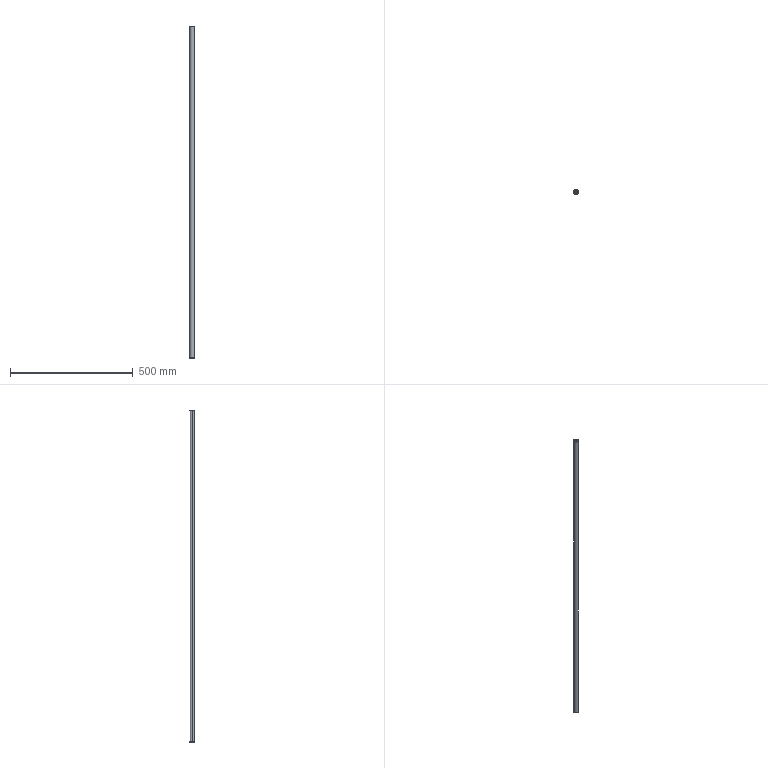Part | STEP file | DCV-000-007 | 1 solid | 16 faces | box 20 x 20 x 1350 mm | volume 418710 mm3 | cone 8 | cylinder 6 | plane 2 | commonest cylinder face diameters 10.106 x4 20 x2
STEP:
#1=CARTESIAN_POINT('',(0.,0.,0.));
#2=DIRECTION('',(0.,0.,1.));
#3=DIRECTION('',(1.,0.,0.));
#4=AXIS2_PLACEMENT_3D('',#1,#2,#3);
#5=CARTESIAN_POINT('',(-9.,0.,675.));
#6=VERTEX_POINT('',#5);
#7=CARTESIAN_POINT('',(9.,0.,675.));
#8=VERTEX_POINT('',#7);
#9=CARTESIAN_POINT('',(0.,0.,675.));
#10=DIRECTION('',(0.,0.,-1.));
#11=DIRECTION('',(-1.,0.,0.));
#12=AXIS2_PLACEMENT_3D('',#9,#10,#11);
#13=CIRCLE('',#12,9.);
#14=CARTESIAN_POINT('',(0.,0.,674.5));
#15=DIRECTION('',(0.,0.,-1.));
#16=DIRECTION('',(-1.,0.,0.));
#17=AXIS2_PLACEMENT_3D('',#14,#15,#16);
#18=CONICAL_SURFACE('',#17,9.5,0.7854);
#19=CARTESIAN_POINT('',(0.,-0.5));
#20=DIRECTION('',(1.,0.));
#21=VECTOR('',#20,1.);
#22=LINE('',#19,#21);
#23=(GEOMETRIC_REPRESENTATION_CONTEXT(2)PARAMETRIC_REPRESENTATION_CONTEXT()REPRESENTATION_CONTEXT('',''));
#24=DEFINITIONAL_REPRESENTATION('',(#22),#23);
#25=PCURVE('',#18,#24);
#26=CARTESIAN_POINT('',(0.,0.,675.));
#27=DIRECTION('',(0.,0.,1.));
#28=DIRECTION('',(1.,0.,0.));
#29=AXIS2_PLACEMENT_3D('',#26,#27,#28);
#30=PLANE('',#29);
#31=CARTESIAN_POINT('',(-9.,0.));
#32=CARTESIAN_POINT('',(-9.,15.588));
#33=CARTESIAN_POINT('',(4.5,7.794));
#34=CARTESIAN_POINT('',(18.,0.));
#35=CARTESIAN_POINT('',(4.5,-7.794));
#36=CARTESIAN_POINT('',(-9.,-15.588));
#37=CARTESIAN_POINT('',(-9.,0.));
#38=(BOUNDED_CURVE()B_SPLINE_CURVE(2,(#31,#32,#33,#34,#35,#36,#37),.UNSPECIFIED.,.T.,.F.)B_SPLINE_CURVE_WITH_KNOTS((1,2,2,2,2,1),(-2.094,0.,2.094,4.189,6.283,8.378),.UNSPECIFIED.)CURVE()GEOMETRIC_REPRESENTATION_ITEM()RATIONAL_B_SPLINE_CURVE((1.,0.5,1.,0.5,1.,0.5,1.))REPRESENTATION_ITEM(''));
#39=(GEOMETRIC_REPRESENTATION_CONTEXT(2)PARAMETRIC_REPRESENTATION_CONTEXT()REPRESENTATION_CONTEXT('',''));
#40=DEFINITIONAL_REPRESENTATION('',(#38),#39);
#41=PCURVE('',#30,#40);
#42=SURFACE_CURVE('',#13,(#25,#41),.PCURVE_S1.);
#43=EDGE_CURVE('',#6,#8,#42,.T.);
#44=ORIENTED_EDGE('',*,*,#43,.T.);
#45=CARTESIAN_POINT('',(10.,0.,674.));
#46=VERTEX_POINT('',#45);
#47=CARTESIAN_POINT('',(9.5,0.,674.5));
#48=DIRECTION('',(0.7071,0.,-0.7071));
#49=VECTOR('',#48,1.);
#50=LINE('',#47,#49);
#51=CARTESIAN_POINT('',(3.142,0.));
#52=DIRECTION('',(0.,1.));
#53=VECTOR('',#52,1.);
#54=LINE('',#51,#53);
#55=(GEOMETRIC_REPRESENTATION_CONTEXT(2)PARAMETRIC_REPRESENTATION_CONTEXT()REPRESENTATION_CONTEXT('',''));
#56=DEFINITIONAL_REPRESENTATION('',(#54),#55);
#57=PCURVE('',#18,#56);
#58=CARTESIAN_POINT('',(0.,0.,674.5));
#59=DIRECTION('',(0.,0.,-1.));
#60=DIRECTION('',(-1.,0.,0.));
#61=AXIS2_PLACEMENT_3D('',#58,#59,#60);
#62=CONICAL_SURFACE('',#61,9.5,0.7854);
#63=CARTESIAN_POINT('',(3.142,0.));
#64=DIRECTION('',(0.,1.));
#65=VECTOR('',#64,1.);
#66=LINE('',#63,#65);
#67=(GEOMETRIC_REPRESENTATION_CONTEXT(2)PARAMETRIC_REPRESENTATION_CONTEXT()REPRESENTATION_CONTEXT('',''));
#68=DEFINITIONAL_REPRESENTATION('',(#66),#67);
#69=PCURVE('',#62,#68);
#70=SURFACE_CURVE('',#50,(#57,#69),.PCURVE_S1.);
#71=EDGE_CURVE('',#8,#46,#70,.T.);
#72=ORIENTED_EDGE('',*,*,#71,.T.);
#73=CARTESIAN_POINT('',(-10.,0.,674.));
#74=VERTEX_POINT('',#73);
#75=CARTESIAN_POINT('',(0.,0.,674.));
#76=DIRECTION('',(0.,0.,1.));
#77=DIRECTION('',(-1.,0.,0.));
#78=AXIS2_PLACEMENT_3D('',#75,#76,#77);
#79=CIRCLE('',#78,10.);
#80=CARTESIAN_POINT('',(6.283,0.5));
#81=DIRECTION('',(-1.,0.));
#82=VECTOR('',#81,1.);
#83=LINE('',#80,#82);
#84=(GEOMETRIC_REPRESENTATION_CONTEXT(2)PARAMETRIC_REPRESENTATION_CONTEXT()REPRESENTATION_CONTEXT('',''));
#85=DEFINITIONAL_REPRESENTATION('',(#83),#84);
#86=PCURVE('',#18,#85);
#87=CARTESIAN_POINT('',(0.,0.,0.));
#88=DIRECTION('',(0.,0.,1.));
#89=DIRECTION('',(1.,0.,0.));
#90=AXIS2_PLACEMENT_3D('',#87,#88,#89);
#91=CYLINDRICAL_SURFACE('',#90,10.);
#92=CARTESIAN_POINT('',(-3.142,674.));
#93=DIRECTION('',(1.,0.));
#94=VECTOR('',#93,1.);
#95=LINE('',#92,#94);
#96=(GEOMETRIC_REPRESENTATION_CONTEXT(2)PARAMETRIC_REPRESENTATION_CONTEXT()REPRESENTATION_CONTEXT('',''));
#97=DEFINITIONAL_REPRESENTATION('',(#95),#96);
#98=PCURVE('',#91,#97);
#99=SURFACE_CURVE('',#79,(#86,#98),.PCURVE_S1.);
#100=EDGE_CURVE('',#46,#74,#99,.T.);
#101=ORIENTED_EDGE('',*,*,#100,.T.);
#102=CARTESIAN_POINT('',(-9.5,0.,674.5));
#103=DIRECTION('',(-0.7071,0.,-0.7071));
#104=VECTOR('',#103,1.);
#105=LINE('',#102,#104);
#106=CARTESIAN_POINT('',(0.,0.));
#107=DIRECTION('',(0.,1.));
#108=VECTOR('',#107,1.);
#109=LINE('',#106,#108);
#110=(GEOMETRIC_REPRESENTATION_CONTEXT(2)PARAMETRIC_REPRESENTATION_CONTEXT()REPRESENTATION_CONTEXT('',''));
#111=DEFINITIONAL_REPRESENTATION('',(#109),#110);
#112=PCURVE('',#18,#111);
#113=CARTESIAN_POINT('',(6.283,0.));
#114=DIRECTION('',(0.,1.));
#115=VECTOR('',#114,1.);
#116=LINE('',#113,#115);
#117=(GEOMETRIC_REPRESENTATION_CONTEXT(2)PARAMETRIC_REPRESENTATION_CONTEXT()REPRESENTATION_CONTEXT('',''));
#118=DEFINITIONAL_REPRESENTATION('',(#116),#117);
#119=PCURVE('',#62,#118);
#120=SURFACE_CURVE('',#105,(#112,#119),.PCURVE_S1.);
#121=EDGE_CURVE('',#6,#74,#120,.T.);
#122=ORIENTED_EDGE('',*,*,#121,.F.);
#123=EDGE_LOOP('',(#44,#72,#101,#122));
#124=FACE_BOUND('',#123,.T.);
#125=ADVANCED_FACE('',(#124),#18,.T.);
#126=CARTESIAN_POINT('',(-10.,0.,-674.));
#127=VERTEX_POINT('',#126);
#128=CARTESIAN_POINT('',(10.,0.,-674.));
#129=VERTEX_POINT('',#128);
#130=CARTESIAN_POINT('',(0.,0.,-674.));
#131=DIRECTION('',(0.,0.,-1.));
#132=DIRECTION('',(-1.,0.,0.));
#133=AXIS2_PLACEMENT_3D('',#130,#131,#132);
#134=CIRCLE('',#133,10.);
#135=CARTESIAN_POINT('',(3.142,-674.));
#136=DIRECTION('',(-1.,0.));
#137=VECTOR('',#136,1.);
#138=LINE('',#135,#137);
#139=(GEOMETRIC_REPRESENTATION_CONTEXT(2)PARAMETRIC_REPRESENTATION_CONTEXT()REPRESENTATION_CONTEXT('',''));
#140=DEFINITIONAL_REPRESENTATION('',(#138),#139);
#141=PCURVE('',#91,#140);
#142=CARTESIAN_POINT('',(0.,0.,-674.5));
#143=DIRECTION('',(0.,0.,1.));
#144=DIRECTION('',(-1.,0.,0.));
#145=AXIS2_PLACEMENT_3D('',#142,#143,#144);
#146=CONICAL_SURFACE('',#145,9.5,0.7854);
#147=CARTESIAN_POINT('',(6.283,0.5));
#148=DIRECTION('',(-1.,0.));
#149=VECTOR('',#148,1.);
#150=LINE('',#147,#149);
#151=(GEOMETRIC_REPRESENTATION_CONTEXT(2)PARAMETRIC_REPRESENTATION_CONTEXT()REPRESENTATION_CONTEXT('',''));
#152=DEFINITIONAL_REPRESENTATION('',(#150),#151);
#153=PCURVE('',#146,#152);
#154=SURFACE_CURVE('',#134,(#141,#153),.PCURVE_S1.);
#155=EDGE_CURVE('',#127,#129,#154,.T.);
#156=ORIENTED_EDGE('',*,*,#155,.F.);
#157=CARTESIAN_POINT('',(-10.,0.,0.));
#158=DIRECTION('',(0.,0.,1.));
#159=VECTOR('',#158,1.);
#160=LINE('',#157,#159);
#161=CARTESIAN_POINT('',(3.142,0.));
#162=DIRECTION('',(0.,1.));
#163=VECTOR('',#162,1.);
#164=LINE('',#161,#163);
#165=(GEOMETRIC_REPRESENTATION_CONTEXT(2)PARAMETRIC_REPRESENTATION_CONTEXT()REPRESENTATION_CONTEXT('',''));
#166=DEFINITIONAL_REPRESENTATION('',(#164),#165);
#167=PCURVE('',#91,#166);
#168=CARTESIAN_POINT('',(0.,0.,0.));
#169=DIRECTION('',(0.,0.,1.));
#170=DIRECTION('',(1.,0.,0.));
#171=AXIS2_PLACEMENT_3D('',#168,#169,#170);
#172=CYLINDRICAL_SURFACE('',#171,10.);
#173=CARTESIAN_POINT('',(3.142,0.));
#174=DIRECTION('',(0.,1.));
#175=VECTOR('',#174,1.);
#176=LINE('',#173,#175);
#177=(GEOMETRIC_REPRESENTATION_CONTEXT(2)PARAMETRIC_REPRESENTATION_CONTEXT()REPRESENTATION_CONTEXT('',''));
#178=DEFINITIONAL_REPRESENTATION('',(#176),#177);
#179=PCURVE('',#172,#178);
#180=SURFACE_CURVE('',#160,(#167,#179),.PCURVE_S1.);
#181=EDGE_CURVE('',#127,#74,#180,.T.);
#182=ORIENTED_EDGE('',*,*,#181,.T.);
#183=ORIENTED_EDGE('',*,*,#100,.F.);
#184=CARTESIAN_POINT('',(10.,0.,0.));
#185=DIRECTION('',(0.,0.,1.));
#186=VECTOR('',#185,1.);
#187=LINE('',#184,#186);
#188=CARTESIAN_POINT('',(0.,0.));
#189=DIRECTION('',(0.,1.));
#190=VECTOR('',#189,1.);
#191=LINE('',#188,#190);
#192=(GEOMETRIC_REPRESENTATION_CONTEXT(2)PARAMETRIC_REPRESENTATION_CONTEXT()REPRESENTATION_CONTEXT('',''));
#193=DEFINITIONAL_REPRESENTATION('',(#191),#192);
#194=PCURVE('',#91,#193);
#195=CARTESIAN_POINT('',(6.283,0.));
#196=DIRECTION('',(0.,1.));
#197=VECTOR('',#196,1.);
#198=LINE('',#195,#197);
#199=(GEOMETRIC_REPRESENTATION_CONTEXT(2)PARAMETRIC_REPRESENTATION_CONTEXT()REPRESENTATION_CONTEXT('',''));
#200=DEFINITIONAL_REPRESENTATION('',(#198),#199);
#201=PCURVE('',#172,#200);
#202=SURFACE_CURVE('',#187,(#194,#201),.PCURVE_S1.);
#203=EDGE_CURVE('',#129,#46,#202,.T.);
#204=ORIENTED_EDGE('',*,*,#203,.F.);
#205=EDGE_LOOP('',(#156,#182,#183,#204));
#206=FACE_BOUND('',#205,.T.);
#207=ADVANCED_FACE('',(#206),#91,.T.);
#208=CARTESIAN_POINT('',(-9.,0.,-675.));
#209=VERTEX_POINT('',#208);
#210=CARTESIAN_POINT('',(9.,0.,-675.));
#211=VERTEX_POINT('',#210);
#212=CARTESIAN_POINT('',(0.,0.,-675.));
#213=DIRECTION('',(0.,0.,1.));
#214=DIRECTION('',(-1.,0.,0.));
#215=AXIS2_PLACEMENT_3D('',#212,#213,#214);
#216=CIRCLE('',#215,9.);
#217=CARTESIAN_POINT('',(0.,0.,-674.5));
#218=DIRECTION('',(0.,0.,1.));
#219=DIRECTION('',(-1.,0.,0.));
#220=AXIS2_PLACEMENT_3D('',#217,#218,#219);
#221=CONICAL_SURFACE('',#220,9.5,0.7854);
#222=CARTESIAN_POINT('',(0.,-0.5));
#223=DIRECTION('',(1.,0.));
#224=VECTOR('',#223,1.);
#225=LINE('',#222,#224);
#226=(GEOMETRIC_REPRESENTATION_CONTEXT(2)PARAMETRIC_REPRESENTATION_CONTEXT()REPRESENTATION_CONTEXT('',''));
#227=DEFINITIONAL_REPRESENTATION('',(#225),#226);
#228=PCURVE('',#221,#227);
#229=CARTESIAN_POINT('',(0.,0.,-675.));
#230=DIRECTION('',(0.,0.,1.));
#231=DIRECTION('',(1.,0.,0.));
#232=AXIS2_PLACEMENT_3D('',#229,#230,#231);
#233=PLANE('',#232);
#234=CARTESIAN_POINT('',(0.,0.));
#235=DIRECTION('',(-1.,0.));
#236=AXIS2_PLACEMENT_2D('',#234,#235);
#237=CIRCLE('',#236,9.);
#238=(GEOMETRIC_REPRESENTATION_CONTEXT(2)PARAMETRIC_REPRESENTATION_CONTEXT()REPRESENTATION_CONTEXT('',''));
#239=DEFINITIONAL_REPRESENTATION('',(#237),#238);
#240=PCURVE('',#233,#239);
#241=SURFACE_CURVE('',#216,(#228,#240),.PCURVE_S1.);
#242=EDGE_CURVE('',#209,#211,#241,.T.);
#243=ORIENTED_EDGE('',*,*,#242,.T.);
#244=CARTESIAN_POINT('',(9.5,0.,-674.5));
#245=DIRECTION('',(0.7071,0.,0.7071));
#246=VECTOR('',#245,1.);
#247=LINE('',#244,#246);
#248=CARTESIAN_POINT('',(3.142,0.));
#249=DIRECTION('',(0.,1.));
#250=VECTOR('',#249,1.);
#251=LINE('',#248,#250);
#252=(GEOMETRIC_REPRESENTATION_CONTEXT(2)PARAMETRIC_REPRESENTATION_CONTEXT()REPRESENTATION_CONTEXT('',''));
#253=DEFINITIONAL_REPRESENTATION('',(#251),#252);
#254=PCURVE('',#221,#253);
#255=CARTESIAN_POINT('',(3.142,0.));
#256=DIRECTION('',(0.,1.));
#257=VECTOR('',#256,1.);
#258=LINE('',#255,#257);
#259=(GEOMETRIC_REPRESENTATION_CONTEXT(2)PARAMETRIC_REPRESENTATION_CONTEXT()REPRESENTATION_CONTEXT('',''));
#260=DEFINITIONAL_REPRESENTATION('',(#258),#259);
#261=PCURVE('',#146,#260);
#262=SURFACE_CURVE('',#247,(#254,#261),.PCURVE_S1.);
#263=EDGE_CURVE('',#211,#129,#262,.T.);
#264=ORIENTED_EDGE('',*,*,#263,.T.);
#265=CARTESIAN_POINT('',(0.,0.,-674.));
#266=DIRECTION('',(0.,0.,-1.));
#267=DIRECTION('',(-1.,0.,0.));
#268=AXIS2_PLACEMENT_3D('',#265,#266,#267);
#269=CIRCLE('',#268,10.);
#270=CARTESIAN_POINT('',(6.283,0.5));
#271=DIRECTION('',(-1.,0.));
#272=VECTOR('',#271,1.);
#273=LINE('',#270,#272);
#274=(GEOMETRIC_REPRESENTATION_CONTEXT(2)PARAMETRIC_REPRESENTATION_CONTEXT()REPRESENTATION_CONTEXT('',''));
#275=DEFINITIONAL_REPRESENTATION('',(#273),#274);
#276=PCURVE('',#221,#275);
#277=CARTESIAN_POINT('',(9.425,-674.));
#278=DIRECTION('',(-1.,0.));
#279=VECTOR('',#278,1.);
#280=LINE('',#277,#279);
#281=(GEOMETRIC_REPRESENTATION_CONTEXT(2)PARAMETRIC_REPRESENTATION_CONTEXT()REPRESENTATION_CONTEXT('',''));
#282=DEFINITIONAL_REPRESENTATION('',(#280),#281);
#283=PCURVE('',#172,#282);
#284=SURFACE_CURVE('',#269,(#276,#283),.PCURVE_S1.);
#285=EDGE_CURVE('',#129,#127,#284,.T.);
#286=ORIENTED_EDGE('',*,*,#285,.T.);
#287=CARTESIAN_POINT('',(-9.5,0.,-674.5));
#288=DIRECTION('',(-0.7071,0.,0.7071));
#289=VECTOR('',#288,1.);
#290=LINE('',#287,#289);
#291=CARTESIAN_POINT('',(0.,0.));
#292=DIRECTION('',(0.,1.));
#293=VECTOR('',#292,1.);
#294=LINE('',#291,#293);
#295=(GEOMETRIC_REPRESENTATION_CONTEXT(2)PARAMETRIC_REPRESENTATION_CONTEXT()REPRESENTATION_CONTEXT('',''));
#296=DEFINITIONAL_REPRESENTATION('',(#294),#295);
#297=PCURVE('',#221,#296);
#298=CARTESIAN_POINT('',(6.283,0.));
#299=DIRECTION('',(0.,1.));
#300=VECTOR('',#299,1.);
#301=LINE('',#298,#300);
#302=(GEOMETRIC_REPRESENTATION_CONTEXT(2)PARAMETRIC_REPRESENTATION_CONTEXT()REPRESENTATION_CONTEXT('',''));
#303=DEFINITIONAL_REPRESENTATION('',(#301),#302);
#304=PCURVE('',#146,#303);
#305=SURFACE_CURVE('',#290,(#297,#304),.PCURVE_S1.);
#306=EDGE_CURVE('',#209,#127,#305,.T.);
#307=ORIENTED_EDGE('',*,*,#306,.F.);
#308=EDGE_LOOP('',(#243,#264,#286,#307));
#309=FACE_BOUND('',#308,.T.);
#310=ADVANCED_FACE('',(#309),#221,.T.);
#311=CARTESIAN_POINT('',(5.053,0.,-642.7));
#312=VERTEX_POINT('',#311);
#313=CARTESIAN_POINT('',(-5.053,0.,-642.7));
#314=VERTEX_POINT('',#313);
#315=CARTESIAN_POINT('',(0.,0.,-642.7));
#316=DIRECTION('',(0.,0.,-1.));
#317=DIRECTION('',(-1.,0.,0.));
#318=AXIS2_PLACEMENT_3D('',#315,#316,#317);
#319=CIRCLE('',#318,5.053);
#320=CARTESIAN_POINT('',(0.,0.,-641.182));
#321=DIRECTION('',(0.,0.,-1.));
#322=DIRECTION('',(-1.,0.,0.));
#323=AXIS2_PLACEMENT_3D('',#320,#321,#322);
#324=CONICAL_SURFACE('',#323,2.526,1.03);
#325=CARTESIAN_POINT('',(0.,1.518));
#326=DIRECTION('',(1.,0.));
#327=VECTOR('',#326,1.);
#328=LINE('',#325,#327);
#329=(GEOMETRIC_REPRESENTATION_CONTEXT(2)PARAMETRIC_REPRESENTATION_CONTEXT()REPRESENTATION_CONTEXT('',''));
#330=DEFINITIONAL_REPRESENTATION('',(#328),#329);
#331=PCURVE('',#324,#330);
#332=CARTESIAN_POINT('',(0.,0.,-658.85));
#333=DIRECTION('',(0.,0.,-1.));
#334=DIRECTION('',(-1.,0.,0.));
#335=AXIS2_PLACEMENT_3D('',#332,#333,#334);
#336=CYLINDRICAL_SURFACE('',#335,5.053);
#337=CARTESIAN_POINT('',(0.,-16.15));
#338=DIRECTION('',(1.,0.));
#339=VECTOR('',#338,1.);
#340=LINE('',#337,#339);
#341=(GEOMETRIC_REPRESENTATION_CONTEXT(2)PARAMETRIC_REPRESENTATION_CONTEXT()REPRESENTATION_CONTEXT('',''));
#342=DEFINITIONAL_REPRESENTATION('',(#340),#341);
#343=PCURVE('',#336,#342);
#344=SURFACE_CURVE('',#319,(#331,#343),.PCURVE_S1.);
#345=EDGE_CURVE('',#312,#314,#344,.T.);
#346=ORIENTED_EDGE('',*,*,#345,.F.);
#347=CARTESIAN_POINT('',(0.,0.,-639.664));
#348=VERTEX_POINT('',#347);
#349=CARTESIAN_POINT('',(2.526,0.,-641.182));
#350=DIRECTION('',(0.8572,0.,-0.515));
#351=VECTOR('',#350,1.);
#352=LINE('',#349,#351);
#353=CARTESIAN_POINT('',(3.142,0.));
#354=DIRECTION('',(0.,1.));
#355=VECTOR('',#354,1.);
#356=LINE('',#353,#355);
#357=(GEOMETRIC_REPRESENTATION_CONTEXT(2)PARAMETRIC_REPRESENTATION_CONTEXT()REPRESENTATION_CONTEXT('',''));
#358=DEFINITIONAL_REPRESENTATION('',(#356),#357);
#359=PCURVE('',#324,#358);
#360=CARTESIAN_POINT('',(0.,0.,-641.182));
#361=DIRECTION('',(0.,0.,-1.));
#362=DIRECTION('',(-1.,0.,0.));
#363=AXIS2_PLACEMENT_3D('',#360,#361,#362);
#364=CONICAL_SURFACE('',#363,2.526,1.03);
#365=CARTESIAN_POINT('',(3.142,0.));
#366=DIRECTION('',(0.,1.));
#367=VECTOR('',#366,1.);
#368=LINE('',#365,#367);
#369=(GEOMETRIC_REPRESENTATION_CONTEXT(2)PARAMETRIC_REPRESENTATION_CONTEXT()REPRESENTATION_CONTEXT('',''));
#370=DEFINITIONAL_REPRESENTATION('',(#368),#369);
#371=PCURVE('',#364,#370);
#372=SURFACE_CURVE('',#352,(#359,#371),.PCURVE_S1.);
#373=EDGE_CURVE('',#348,#312,#372,.T.);
#374=ORIENTED_EDGE('',*,*,#373,.F.);
#375=CARTESIAN_POINT('',(-2.526,0.,-641.182));
#376=DIRECTION('',(-0.8572,0.,-0.515));
#377=VECTOR('',#376,1.);
#378=LINE('',#375,#377);
#379=CARTESIAN_POINT('',(6.283,0.));
#380=DIRECTION('',(0.,1.));
#381=VECTOR('',#380,1.);
#382=LINE('',#379,#381);
#383=(GEOMETRIC_REPRESENTATION_CONTEXT(2)PARAMETRIC_REPRESENTATION_CONTEXT()REPRESENTATION_CONTEXT('',''));
#384=DEFINITIONAL_REPRESENTATION('',(#382),#383);
#385=PCURVE('',#324,#384);
#386=CARTESIAN_POINT('',(0.,0.));
#387=DIRECTION('',(0.,1.));
#388=VECTOR('',#387,1.);
#389=LINE('',#386,#388);
#390=(GEOMETRIC_REPRESENTATION_CONTEXT(2)PARAMETRIC_REPRESENTATION_CONTEXT()REPRESENTATION_CONTEXT('',''));
#391=DEFINITIONAL_REPRESENTATION('',(#389),#390);
#392=PCURVE('',#364,#391);
#393=SURFACE_CURVE('',#378,(#385,#392),.PCURVE_S1.);
#394=EDGE_CURVE('',#348,#314,#393,.T.);
#395=ORIENTED_EDGE('',*,*,#394,.T.);
#396=EDGE_LOOP('',(#346,#374,#395));
#397=FACE_BOUND('',#396,.F.);
#398=ADVANCED_FACE('',(#397),#324,.F.);
#399=CARTESIAN_POINT('',(-5.053,0.,-675.));
#400=VERTEX_POINT('',#399);
#401=CARTESIAN_POINT('',(-5.053,0.,-658.85));
#402=DIRECTION('',(0.,0.,-1.));
#403=VECTOR('',#402,1.);
#404=LINE('',#401,#403);
#405=CARTESIAN_POINT('',(6.283,0.));
#406=DIRECTION('',(0.,1.));
#407=VECTOR('',#406,1.);
#408=LINE('',#405,#407);
#409=(GEOMETRIC_REPRESENTATION_CONTEXT(2)PARAMETRIC_REPRESENTATION_CONTEXT()REPRESENTATION_CONTEXT('',''));
#410=DEFINITIONAL_REPRESENTATION('',(#408),#409);
#411=PCURVE('',#336,#410);
#412=CARTESIAN_POINT('',(0.,0.,-658.85));
#413=DIRECTION('',(0.,0.,-1.));
#414=DIRECTION('',(-1.,0.,0.));
#415=AXIS2_PLACEMENT_3D('',#412,#413,#414);
#416=CYLINDRICAL_SURFACE('',#415,5.053);
#417=CARTESIAN_POINT('',(0.,0.));
#418=DIRECTION('',(0.,1.));
#419=VECTOR('',#418,1.);
#420=LINE('',#417,#419);
#421=(GEOMETRIC_REPRESENTATION_CONTEXT(2)PARAMETRIC_REPRESENTATION_CONTEXT()REPRESENTATION_CONTEXT('',''));
#422=DEFINITIONAL_REPRESENTATION('',(#420),#421);
#423=PCURVE('',#416,#422);
#424=SURFACE_CURVE('',#404,(#411,#423),.PCURVE_S1.);
#425=EDGE_CURVE('',#314,#400,#424,.T.);
#426=ORIENTED_EDGE('',*,*,#425,.T.);
#427=CARTESIAN_POINT('',(5.053,0.,-675.));
#428=VERTEX_POINT('',#427);
#429=CARTESIAN_POINT('',(0.,0.,-675.));
#430=DIRECTION('',(0.,0.,1.));
#431=DIRECTION('',(-1.,0.,0.));
#432=AXIS2_PLACEMENT_3D('',#429,#430,#431);
#433=CIRCLE('',#432,5.053);
#434=CARTESIAN_POINT('',(6.283,16.15));
#435=DIRECTION('',(-1.,0.));
#436=VECTOR('',#435,1.);
#437=LINE('',#434,#436);
#438=(GEOMETRIC_REPRESENTATION_CONTEXT(2)PARAMETRIC_REPRESENTATION_CONTEXT()REPRESENTATION_CONTEXT('',''));
#439=DEFINITIONAL_REPRESENTATION('',(#437),#438);
#440=PCURVE('',#336,#439);
#441=CARTESIAN_POINT('',(0.,0.));
#442=DIRECTION('',(-1.,0.));
#443=AXIS2_PLACEMENT_2D('',#441,#442);
#444=CIRCLE('',#443,5.053);
#445=(GEOMETRIC_REPRESENTATION_CONTEXT(2)PARAMETRIC_REPRESENTATION_CONTEXT()REPRESENTATION_CONTEXT('',''));
#446=DEFINITIONAL_REPRESENTATION('',(#444),#445);
#447=PCURVE('',#233,#446);
#448=SURFACE_CURVE('',#433,(#440,#447),.PCURVE_S1.);
#449=EDGE_CURVE('',#400,#428,#448,.T.);
#450=ORIENTED_EDGE('',*,*,#449,.T.);
#451=CARTESIAN_POINT('',(5.053,0.,-658.85));
#452=DIRECTION('',(0.,0.,-1.));
#453=VECTOR('',#452,1.);
#454=LINE('',#451,#453);
#455=CARTESIAN_POINT('',(3.142,0.));
#456=DIRECTION('',(0.,1.));
#457=VECTOR('',#456,1.);
#458=LINE('',#455,#457);
#459=(GEOMETRIC_REPRESENTATION_CONTEXT(2)PARAMETRIC_REPRESENTATION_CONTEXT()REPRESENTATION_CONTEXT('',''));
#460=DEFINITIONAL_REPRESENTATION('',(#458),#459);
#461=PCURVE('',#336,#460);
#462=CARTESIAN_POINT('',(3.142,0.));
#463=DIRECTION('',(0.,1.));
#464=VECTOR('',#463,1.);
#465=LINE('',#462,#464);
#466=(GEOMETRIC_REPRESENTATION_CONTEXT(2)PARAMETRIC_REPRESENTATION_CONTEXT()REPRESENTATION_CONTEXT('',''));
#467=DEFINITIONAL_REPRESENTATION('',(#465),#466);
#468=PCURVE('',#416,#467);
#469=SURFACE_CURVE('',#454,(#461,#468),.PCURVE_S1.);
#470=EDGE_CURVE('',#312,#428,#469,.T.);
#471=ORIENTED_EDGE('',*,*,#470,.F.);
#472=ORIENTED_EDGE('',*,*,#345,.T.);
#473=EDGE_LOOP('',(#426,#450,#471,#472));
#474=FACE_BOUND('',#473,.F.);
#475=ADVANCED_FACE('',(#474),#336,.F.);
#476=CARTESIAN_POINT('',(-5.053,0.,642.7));
#477=VERTEX_POINT('',#476);
#478=CARTESIAN_POINT('',(5.053,0.,642.7));
#479=VERTEX_POINT('',#478);
#480=CARTESIAN_POINT('',(0.,0.,642.7));
#481=DIRECTION('',(0.,0.,1.));
#482=DIRECTION('',(1.,0.,0.));
#483=AXIS2_PLACEMENT_3D('',#480,#481,#482);
#484=CIRCLE('',#483,5.053);
#485=CARTESIAN_POINT('',(0.,0.,641.182));
#486=DIRECTION('',(0.,0.,1.));
#487=DIRECTION('',(1.,0.,0.));
#488=AXIS2_PLACEMENT_3D('',#485,#486,#487);
#489=CONICAL_SURFACE('',#488,2.526,1.03);
#490=CARTESIAN_POINT('',(0.,1.518));
#491=DIRECTION('',(1.,0.));
#492=VECTOR('',#491,1.);
#493=LINE('',#490,#492);
#494=(GEOMETRIC_REPRESENTATION_CONTEXT(2)PARAMETRIC_REPRESENTATION_CONTEXT()REPRESENTATION_CONTEXT('',''));
#495=DEFINITIONAL_REPRESENTATION('',(#493),#494);
#496=PCURVE('',#489,#495);
#497=CARTESIAN_POINT('',(0.,0.,658.85));
#498=DIRECTION('',(0.,0.,1.));
#499=DIRECTION('',(1.,0.,0.));
#500=AXIS2_PLACEMENT_3D('',#497,#498,#499);
#501=CYLINDRICAL_SURFACE('',#500,5.053);
#502=CARTESIAN_POINT('',(0.,-16.15));
#503=DIRECTION('',(1.,0.));
#504=VECTOR('',#503,1.);
#505=LINE('',#502,#504);
#506=(GEOMETRIC_REPRESENTATION_CONTEXT(2)PARAMETRIC_REPRESENTATION_CONTEXT()REPRESENTATION_CONTEXT('',''));
#507=DEFINITIONAL_REPRESENTATION('',(#505),#506);
#508=PCURVE('',#501,#507);
#509=SURFACE_CURVE('',#484,(#496,#508),.PCURVE_S1.);
#510=EDGE_CURVE('',#477,#479,#509,.T.);
#511=ORIENTED_EDGE('',*,*,#510,.F.);
#512=CARTESIAN_POINT('',(0.,0.,639.664));
#513=VERTEX_POINT('',#512);
#514=CARTESIAN_POINT('',(-2.526,0.,641.182));
#515=DIRECTION('',(-0.8572,0.,0.515));
#516=VECTOR('',#515,1.);
#517=LINE('',#514,#516);
#518=CARTESIAN_POINT('',(3.142,0.));
#519=DIRECTION('',(0.,1.));
#520=VECTOR('',#519,1.);
#521=LINE('',#518,#520);
#522=(GEOMETRIC_REPRESENTATION_CONTEXT(2)PARAMETRIC_REPRESENTATION_CONTEXT()REPRESENTATION_CONTEXT('',''));
#523=DEFINITIONAL_REPRESENTATION('',(#521),#522);
#524=PCURVE('',#489,#523);
#525=CARTESIAN_POINT('',(0.,0.,641.182));
#526=DIRECTION('',(0.,0.,1.));
#527=DIRECTION('',(1.,0.,0.));
#528=AXIS2_PLACEMENT_3D('',#525,#526,#527);
#529=CONICAL_SURFACE('',#528,2.526,1.03);
#530=CARTESIAN_POINT('',(3.142,0.));
#531=DIRECTION('',(0.,1.));
#532=VECTOR('',#531,1.);
#533=LINE('',#530,#532);
#534=(GEOMETRIC_REPRESENTATION_CONTEXT(2)PARAMETRIC_REPRESENTATION_CONTEXT()REPRESENTATION_CONTEXT('',''));
#535=DEFINITIONAL_REPRESENTATION('',(#533),#534);
#536=PCURVE('',#529,#535);
#537=SURFACE_CURVE('',#517,(#524,#536),.PCURVE_S1.);
#538=EDGE_CURVE('',#513,#477,#537,.T.);
#539=ORIENTED_EDGE('',*,*,#538,.F.);
#540=CARTESIAN_POINT('',(2.526,0.,641.182));
#541=DIRECTION('',(0.8572,0.,0.515));
#542=VECTOR('',#541,1.);
#543=LINE('',#540,#542);
#544=CARTESIAN_POINT('',(6.283,0.));
#545=DIRECTION('',(0.,1.));
#546=VECTOR('',#545,1.);
#547=LINE('',#544,#546);
#548=(GEOMETRIC_REPRESENTATION_CONTEXT(2)PARAMETRIC_REPRESENTATION_CONTEXT()REPRESENTATION_CONTEXT('',''));
#549=DEFINITIONAL_REPRESENTATION('',(#547),#548);
#550=PCURVE('',#489,#549);
#551=CARTESIAN_POINT('',(0.,0.));
#552=DIRECTION('',(0.,1.));
#553=VECTOR('',#552,1.);
#554=LINE('',#551,#553);
#555=(GEOMETRIC_REPRESENTATION_CONTEXT(2)PARAMETRIC_REPRESENTATION_CONTEXT()REPRESENTATION_CONTEXT('',''));
#556=DEFINITIONAL_REPRESENTATION('',(#554),#555);
#557=PCURVE('',#529,#556);
#558=SURFACE_CURVE('',#543,(#550,#557),.PCURVE_S1.);
#559=EDGE_CURVE('',#513,#479,#558,.T.);
#560=ORIENTED_EDGE('',*,*,#559,.T.);
#561=EDGE_LOOP('',(#511,#539,#560));
#562=FACE_BOUND('',#561,.F.);
#563=ADVANCED_FACE('',(#562),#489,.F.);
#564=CARTESIAN_POINT('',(5.053,0.,675.));
#565=VERTEX_POINT('',#564);
#566=CARTESIAN_POINT('',(5.053,0.,658.85));
#567=DIRECTION('',(0.,0.,1.));
#568=VECTOR('',#567,1.);
#569=LINE('',#566,#568);
#570=CARTESIAN_POINT('',(6.283,0.));
#571=DIRECTION('',(0.,1.));
#572=VECTOR('',#571,1.);
#573=LINE('',#570,#572);
#574=(GEOMETRIC_REPRESENTATION_CONTEXT(2)PARAMETRIC_REPRESENTATION_CONTEXT()REPRESENTATION_CONTEXT('',''));
#575=DEFINITIONAL_REPRESENTATION('',(#573),#574);
#576=PCURVE('',#501,#575);
#577=CARTESIAN_POINT('',(0.,0.,658.85));
#578=DIRECTION('',(0.,0.,1.));
#579=DIRECTION('',(1.,0.,0.));
#580=AXIS2_PLACEMENT_3D('',#577,#578,#579);
#581=CYLINDRICAL_SURFACE('',#580,5.053);
#582=CARTESIAN_POINT('',(0.,0.));
#583=DIRECTION('',(0.,1.));
#584=VECTOR('',#583,1.);
#585=LINE('',#582,#584);
#586=(GEOMETRIC_REPRESENTATION_CONTEXT(2)PARAMETRIC_REPRESENTATION_CONTEXT()REPRESENTATION_CONTEXT('',''));
#587=DEFINITIONAL_REPRESENTATION('',(#585),#586);
#588=PCURVE('',#581,#587);
#589=SURFACE_CURVE('',#569,(#576,#588),.PCURVE_S1.);
#590=EDGE_CURVE('',#479,#565,#589,.T.);
#591=ORIENTED_EDGE('',*,*,#590,.T.);
#592=CARTESIAN_POINT('',(-5.053,0.,675.));
#593=VERTEX_POINT('',#592);
#594=CARTESIAN_POINT('',(0.,0.,675.));
#595=DIRECTION('',(0.,0.,-1.));
#596=DIRECTION('',(1.,0.,0.));
#597=AXIS2_PLACEMENT_3D('',#594,#595,#596);
#598=CIRCLE('',#597,5.053);
#599=CARTESIAN_POINT('',(6.283,16.15));
#600=DIRECTION('',(-1.,0.));
#601=VECTOR('',#600,1.);
#602=LINE('',#599,#601);
#603=(GEOMETRIC_REPRESENTATION_CONTEXT(2)PARAMETRIC_REPRESENTATION_CONTEXT()REPRESENTATION_CONTEXT('',''));
#604=DEFINITIONAL_REPRESENTATION('',(#602),#603);
#605=PCURVE('',#501,#604);
#606=CARTESIAN_POINT('',(5.053,0.));
#607=CARTESIAN_POINT('',(5.053,-8.752));
#608=CARTESIAN_POINT('',(-2.526,-4.376));
#609=CARTESIAN_POINT('',(-10.106,0.));
#610=CARTESIAN_POINT('',(-2.526,4.376));
#611=CARTESIAN_POINT('',(5.053,8.752));
#612=CARTESIAN_POINT('',(5.053,0.));
#613=(BOUNDED_CURVE()B_SPLINE_CURVE(2,(#606,#607,#608,#609,#610,#611,#612),.UNSPECIFIED.,.T.,.F.)B_SPLINE_CURVE_WITH_KNOTS((1,2,2,2,2,1),(-2.094,0.,2.094,4.189,6.283,8.378),.UNSPECIFIED.)CURVE()GEOMETRIC_REPRESENTATION_ITEM()RATIONAL_B_SPLINE_CURVE((1.,0.5,1.,0.5,1.,0.5,1.))REPRESENTATION_ITEM(''));
#614=(GEOMETRIC_REPRESENTATION_CONTEXT(2)PARAMETRIC_REPRESENTATION_CONTEXT()REPRESENTATION_CONTEXT('',''));
#615=DEFINITIONAL_REPRESENTATION('',(#613),#614);
#616=PCURVE('',#30,#615);
#617=SURFACE_CURVE('',#598,(#605,#616),.PCURVE_S1.);
#618=EDGE_CURVE('',#565,#593,#617,.T.);
#619=ORIENTED_EDGE('',*,*,#618,.T.);
#620=CARTESIAN_POINT('',(-5.053,0.,658.85));
#621=DIRECTION('',(0.,0.,1.));
#622=VECTOR('',#621,1.);
#623=LINE('',#620,#622);
#624=CARTESIAN_POINT('',(3.142,0.));
#625=DIRECTION('',(0.,1.));
#626=VECTOR('',#625,1.);
#627=LINE('',#624,#626);
#628=(GEOMETRIC_REPRESENTATION_CONTEXT(2)PARAMETRIC_REPRESENTATION_CONTEXT()REPRESENTATION_CONTEXT('',''));
#629=DEFINITIONAL_REPRESENTATION('',(#627),#628);
#630=PCURVE('',#501,#629);
#631=CARTESIAN_POINT('',(3.142,0.));
#632=DIRECTION('',(0.,1.));
#633=VECTOR('',#632,1.);
#634=LINE('',#631,#633);
#635=(GEOMETRIC_REPRESENTATION_CONTEXT(2)PARAMETRIC_REPRESENTATION_CONTEXT()REPRESENTATION_CONTEXT('',''));
#636=DEFINITIONAL_REPRESENTATION('',(#634),#635);
#637=PCURVE('',#581,#636);
#638=SURFACE_CURVE('',#623,(#630,#637),.PCURVE_S1.);
#639=EDGE_CURVE('',#477,#593,#638,.T.);
#640=ORIENTED_EDGE('',*,*,#639,.F.);
#641=ORIENTED_EDGE('',*,*,#510,.T.);
#642=EDGE_LOOP('',(#591,#619,#640,#641));
#643=FACE_BOUND('',#642,.F.);
#644=ADVANCED_FACE('',(#643),#501,.F.);
#645=CARTESIAN_POINT('',(0.,0.,675.));
#646=DIRECTION('',(0.,0.,-1.));
#647=DIRECTION('',(1.,0.,0.));
#648=AXIS2_PLACEMENT_3D('',#645,#646,#647);
#649=CIRCLE('',#648,5.053);
#650=CARTESIAN_POINT('',(6.283,16.15));
#651=DIRECTION('',(-1.,0.));
#652=VECTOR('',#651,1.);
#653=LINE('',#650,#652);
#654=(GEOMETRIC_REPRESENTATION_CONTEXT(2)PARAMETRIC_REPRESENTATION_CONTEXT()REPRESENTATION_CONTEXT('',''));
#655=DEFINITIONAL_REPRESENTATION('',(#653),#654);
#656=PCURVE('',#581,#655);
#657=CARTESIAN_POINT('',(5.053,0.));
#658=CARTESIAN_POINT('',(5.053,-8.752));
#659=CARTESIAN_POINT('',(-2.526,-4.376));
#660=CARTESIAN_POINT('',(-10.106,0.));
#661=CARTESIAN_POINT('',(-2.526,4.376));
#662=CARTESIAN_POINT('',(5.053,8.752));
#663=CARTESIAN_POINT('',(5.053,0.));
#664=(BOUNDED_CURVE()B_SPLINE_CURVE(2,(#657,#658,#659,#660,#661,#662,#663),.UNSPECIFIED.,.T.,.F.)B_SPLINE_CURVE_WITH_KNOTS((1,2,2,2,2,1),(-2.094,0.,2.094,4.189,6.283,8.378),.UNSPECIFIED.)CURVE()GEOMETRIC_REPRESENTATION_ITEM()RATIONAL_B_SPLINE_CURVE((1.,0.5,1.,0.5,1.,0.5,1.))REPRESENTATION_ITEM(''));
#665=(GEOMETRIC_REPRESENTATION_CONTEXT(2)PARAMETRIC_REPRESENTATION_CONTEXT()REPRESENTATION_CONTEXT('',''));
#666=DEFINITIONAL_REPRESENTATION('',(#664),#665);
#667=PCURVE('',#30,#666);
#668=SURFACE_CURVE('',#649,(#656,#667),.PCURVE_S1.);
#669=EDGE_CURVE('',#593,#565,#668,.T.);
#670=ORIENTED_EDGE('',*,*,#669,.T.);
#671=ORIENTED_EDGE('',*,*,#590,.F.);
#672=CARTESIAN_POINT('',(0.,0.,642.7));
#673=DIRECTION('',(0.,0.,1.));
#674=DIRECTION('',(1.,0.,0.));
#675=AXIS2_PLACEMENT_3D('',#672,#673,#674);
#676=CIRCLE('',#675,5.053);
#677=CARTESIAN_POINT('',(0.,-16.15));
#678=DIRECTION('',(1.,0.));
#679=VECTOR('',#678,1.);
#680=LINE('',#677,#679);
#681=(GEOMETRIC_REPRESENTATION_CONTEXT(2)PARAMETRIC_REPRESENTATION_CONTEXT()REPRESENTATION_CONTEXT('',''));
#682=DEFINITIONAL_REPRESENTATION('',(#680),#681);
#683=PCURVE('',#581,#682);
#684=CARTESIAN_POINT('',(0.,1.518));
#685=DIRECTION('',(1.,0.));
#686=VECTOR('',#685,1.);
#687=LINE('',#684,#686);
#688=(GEOMETRIC_REPRESENTATION_CONTEXT(2)PARAMETRIC_REPRESENTATION_CONTEXT()REPRESENTATION_CONTEXT('',''));
#689=DEFINITIONAL_REPRESENTATION('',(#687),#688);
#690=PCURVE('',#529,#689);
#691=SURFACE_CURVE('',#676,(#683,#690),.PCURVE_S1.);
#692=EDGE_CURVE('',#479,#477,#691,.T.);
#693=ORIENTED_EDGE('',*,*,#692,.T.);
#694=ORIENTED_EDGE('',*,*,#639,.T.);
#695=EDGE_LOOP('',(#670,#671,#693,#694));
#696=FACE_BOUND('',#695,.F.);
#697=ADVANCED_FACE('',(#696),#581,.F.);
#698=ORIENTED_EDGE('',*,*,#692,.F.);
#699=ORIENTED_EDGE('',*,*,#559,.F.);
#700=ORIENTED_EDGE('',*,*,#538,.T.);
#701=EDGE_LOOP('',(#698,#699,#700));
#702=FACE_BOUND('',#701,.F.);
#703=ADVANCED_FACE('',(#702),#529,.F.);
#704=CARTESIAN_POINT('',(0.,0.,-675.));
#705=DIRECTION('',(0.,0.,1.));
#706=DIRECTION('',(-1.,0.,0.));
#707=AXIS2_PLACEMENT_3D('',#704,#705,#706);
#708=CIRCLE('',#707,5.053);
#709=CARTESIAN_POINT('',(6.283,16.15));
#710=DIRECTION('',(-1.,0.));
#711=VECTOR('',#710,1.);
#712=LINE('',#709,#711);
#713=(GEOMETRIC_REPRESENTATION_CONTEXT(2)PARAMETRIC_REPRESENTATION_CONTEXT()REPRESENTATION_CONTEXT('',''));
#714=DEFINITIONAL_REPRESENTATION('',(#712),#713);
#715=PCURVE('',#416,#714);
#716=CARTESIAN_POINT('',(0.,0.));
#717=DIRECTION('',(-1.,0.));
#718=AXIS2_PLACEMENT_2D('',#716,#717);
#719=CIRCLE('',#718,5.053);
#720=(GEOMETRIC_REPRESENTATION_CONTEXT(2)PARAMETRIC_REPRESENTATION_CONTEXT()REPRESENTATION_CONTEXT('',''));
#721=DEFINITIONAL_REPRESENTATION('',(#719),#720);
#722=PCURVE('',#233,#721);
#723=SURFACE_CURVE('',#708,(#715,#722),.PCURVE_S1.);
#724=EDGE_CURVE('',#428,#400,#723,.T.);
#725=ORIENTED_EDGE('',*,*,#724,.T.);
#726=ORIENTED_EDGE('',*,*,#425,.F.);
#727=CARTESIAN_POINT('',(0.,0.,-642.7));
#728=DIRECTION('',(0.,0.,-1.));
#729=DIRECTION('',(-1.,0.,0.));
#730=AXIS2_PLACEMENT_3D('',#727,#728,#729);
#731=CIRCLE('',#730,5.053);
#732=CARTESIAN_POINT('',(0.,-16.15));
#733=DIRECTION('',(1.,0.));
#734=VECTOR('',#733,1.);
#735=LINE('',#732,#734);
#736=(GEOMETRIC_REPRESENTATION_CONTEXT(2)PARAMETRIC_REPRESENTATION_CONTEXT()REPRESENTATION_CONTEXT('',''));
#737=DEFINITIONAL_REPRESENTATION('',(#735),#736);
#738=PCURVE('',#416,#737);
#739=CARTESIAN_POINT('',(0.,1.518));
#740=DIRECTION('',(1.,0.));
#741=VECTOR('',#740,1.);
#742=LINE('',#739,#741);
#743=(GEOMETRIC_REPRESENTATION_CONTEXT(2)PARAMETRIC_REPRESENTATION_CONTEXT()REPRESENTATION_CONTEXT('',''));
#744=DEFINITIONAL_REPRESENTATION('',(#742),#743);
#745=PCURVE('',#364,#744);
#746=SURFACE_CURVE('',#731,(#738,#745),.PCURVE_S1.);
#747=EDGE_CURVE('',#314,#312,#746,.T.);
#748=ORIENTED_EDGE('',*,*,#747,.T.);
#749=ORIENTED_EDGE('',*,*,#470,.T.);
#750=EDGE_LOOP('',(#725,#726,#748,#749));
#751=FACE_BOUND('',#750,.F.);
#752=ADVANCED_FACE('',(#751),#416,.F.);
#753=ORIENTED_EDGE('',*,*,#747,.F.);
#754=ORIENTED_EDGE('',*,*,#394,.F.);
#755=ORIENTED_EDGE('',*,*,#373,.T.);
#756=EDGE_LOOP('',(#753,#754,#755));
#757=FACE_BOUND('',#756,.F.);
#758=ADVANCED_FACE('',(#757),#364,.F.);
#759=ORIENTED_EDGE('',*,*,#449,.T.);
#760=ORIENTED_EDGE('',*,*,#724,.T.);
#761=EDGE_LOOP('',(#759,#760));
#762=FACE_BOUND('',#761,.T.);
#763=ORIENTED_EDGE('',*,*,#242,.F.);
#764=CARTESIAN_POINT('',(0.,0.,-675.));
#765=DIRECTION('',(0.,0.,1.));
#766=DIRECTION('',(-1.,0.,0.));
#767=AXIS2_PLACEMENT_3D('',#764,#765,#766);
#768=CIRCLE('',#767,9.);
#769=CARTESIAN_POINT('',(0.,0.));
#770=DIRECTION('',(-1.,0.));
#771=AXIS2_PLACEMENT_2D('',#769,#770);
#772=CIRCLE('',#771,9.);
#773=(GEOMETRIC_REPRESENTATION_CONTEXT(2)PARAMETRIC_REPRESENTATION_CONTEXT()REPRESENTATION_CONTEXT('',''));
#774=DEFINITIONAL_REPRESENTATION('',(#772),#773);
#775=PCURVE('',#233,#774);
#776=CARTESIAN_POINT('',(0.,-0.5));
#777=DIRECTION('',(1.,0.));
#778=VECTOR('',#777,1.);
#779=LINE('',#776,#778);
#780=(GEOMETRIC_REPRESENTATION_CONTEXT(2)PARAMETRIC_REPRESENTATION_CONTEXT()REPRESENTATION_CONTEXT('',''));
#781=DEFINITIONAL_REPRESENTATION('',(#779),#780);
#782=PCURVE('',#146,#781);
#783=SURFACE_CURVE('',#768,(#775,#782),.PCURVE_S1.);
#784=EDGE_CURVE('',#211,#209,#783,.T.);
#785=ORIENTED_EDGE('',*,*,#784,.F.);
#786=EDGE_LOOP('',(#763,#785));
#787=FACE_BOUND('',#786,.T.);
#788=ADVANCED_FACE('',(#762,#787),#233,.F.);
#789=ORIENTED_EDGE('',*,*,#263,.F.);
#790=ORIENTED_EDGE('',*,*,#784,.T.);
#791=ORIENTED_EDGE('',*,*,#306,.T.);
#792=ORIENTED_EDGE('',*,*,#155,.T.);
#793=EDGE_LOOP('',(#789,#790,#791,#792));
#794=FACE_BOUND('',#793,.T.);
#795=ADVANCED_FACE('',(#794),#146,.T.);
#796=ORIENTED_EDGE('',*,*,#618,.T.);
#797=ORIENTED_EDGE('',*,*,#669,.T.);
#798=EDGE_LOOP('',(#796,#797));
#799=FACE_BOUND('',#798,.T.);
#800=ORIENTED_EDGE('',*,*,#43,.F.);
#801=CARTESIAN_POINT('',(0.,0.,675.));
#802=DIRECTION('',(0.,0.,-1.));
#803=DIRECTION('',(-1.,0.,0.));
#804=AXIS2_PLACEMENT_3D('',#801,#802,#803);
#805=CIRCLE('',#804,9.);
#806=CARTESIAN_POINT('',(-9.,0.));
#807=CARTESIAN_POINT('',(-9.,15.588));
#808=CARTESIAN_POINT('',(4.5,7.794));
#809=CARTESIAN_POINT('',(18.,0.));
#810=CARTESIAN_POINT('',(4.5,-7.794));
#811=CARTESIAN_POINT('',(-9.,-15.588));
#812=CARTESIAN_POINT('',(-9.,0.));
#813=(BOUNDED_CURVE()B_SPLINE_CURVE(2,(#806,#807,#808,#809,#810,#811,#812),.UNSPECIFIED.,.T.,.F.)B_SPLINE_CURVE_WITH_KNOTS((1,2,2,2,2,1),(-2.094,0.,2.094,4.189,6.283,8.378),.UNSPECIFIED.)CURVE()GEOMETRIC_REPRESENTATION_ITEM()RATIONAL_B_SPLINE_CURVE((1.,0.5,1.,0.5,1.,0.5,1.))REPRESENTATION_ITEM(''));
#814=(GEOMETRIC_REPRESENTATION_CONTEXT(2)PARAMETRIC_REPRESENTATION_CONTEXT()REPRESENTATION_CONTEXT('',''));
#815=DEFINITIONAL_REPRESENTATION('',(#813),#814);
#816=PCURVE('',#30,#815);
#817=CARTESIAN_POINT('',(0.,-0.5));
#818=DIRECTION('',(1.,0.));
#819=VECTOR('',#818,1.);
#820=LINE('',#817,#819);
#821=(GEOMETRIC_REPRESENTATION_CONTEXT(2)PARAMETRIC_REPRESENTATION_CONTEXT()REPRESENTATION_CONTEXT('',''));
#822=DEFINITIONAL_REPRESENTATION('',(#820),#821);
#823=PCURVE('',#62,#822);
#824=SURFACE_CURVE('',#805,(#816,#823),.PCURVE_S1.);
#825=EDGE_CURVE('',#8,#6,#824,.T.);
#826=ORIENTED_EDGE('',*,*,#825,.F.);
#827=EDGE_LOOP('',(#800,#826));
#828=FACE_BOUND('',#827,.T.);
#829=ADVANCED_FACE('',(#799,#828),#30,.T.);
#830=ORIENTED_EDGE('',*,*,#181,.F.);
#831=ORIENTED_EDGE('',*,*,#285,.F.);
#832=ORIENTED_EDGE('',*,*,#203,.T.);
#833=CARTESIAN_POINT('',(0.,0.,674.));
#834=DIRECTION('',(0.,0.,1.));
#835=DIRECTION('',(-1.,0.,0.));
#836=AXIS2_PLACEMENT_3D('',#833,#834,#835);
#837=CIRCLE('',#836,10.);
#838=CARTESIAN_POINT('',(3.142,674.));
#839=DIRECTION('',(1.,0.));
#840=VECTOR('',#839,1.);
#841=LINE('',#838,#840);
#842=(GEOMETRIC_REPRESENTATION_CONTEXT(2)PARAMETRIC_REPRESENTATION_CONTEXT()REPRESENTATION_CONTEXT('',''));
#843=DEFINITIONAL_REPRESENTATION('',(#841),#842);
#844=PCURVE('',#172,#843);
#845=CARTESIAN_POINT('',(6.283,0.5));
#846=DIRECTION('',(-1.,0.));
#847=VECTOR('',#846,1.);
#848=LINE('',#845,#847);
#849=(GEOMETRIC_REPRESENTATION_CONTEXT(2)PARAMETRIC_REPRESENTATION_CONTEXT()REPRESENTATION_CONTEXT('',''));
#850=DEFINITIONAL_REPRESENTATION('',(#848),#849);
#851=PCURVE('',#62,#850);
#852=SURFACE_CURVE('',#837,(#844,#851),.PCURVE_S1.);
#853=EDGE_CURVE('',#74,#46,#852,.T.);
#854=ORIENTED_EDGE('',*,*,#853,.F.);
#855=EDGE_LOOP('',(#830,#831,#832,#854));
#856=FACE_BOUND('',#855,.T.);
#857=ADVANCED_FACE('',(#856),#172,.T.);
#858=ORIENTED_EDGE('',*,*,#71,.F.);
#859=ORIENTED_EDGE('',*,*,#825,.T.);
#860=ORIENTED_EDGE('',*,*,#121,.T.);
#861=ORIENTED_EDGE('',*,*,#853,.T.);
#862=EDGE_LOOP('',(#858,#859,#860,#861));
#863=FACE_BOUND('',#862,.T.);
#864=ADVANCED_FACE('',(#863),#62,.T.);
#865=CLOSED_SHELL('',(#125,#207,#310,#398,#475,#563,#644,#697,#703,#752,#758,#788,#795,#829,#857,#864));
#866=MANIFOLD_SOLID_BREP('',#865);
#867=(LENGTH_UNIT()NAMED_UNIT(*)SI_UNIT(.MILLI.,.METRE.));
#868=UNCERTAINTY_MEASURE_WITH_UNIT(LENGTH_MEASURE(0.0000001),#867,'','');
#869=(NAMED_UNIT(*)PLANE_ANGLE_UNIT()SI_UNIT($,.RADIAN.));
#870=(NAMED_UNIT(*)SI_UNIT($,.STERADIAN.)SOLID_ANGLE_UNIT());
#871=(GEOMETRIC_REPRESENTATION_CONTEXT(3)GLOBAL_UNCERTAINTY_ASSIGNED_CONTEXT((#868))GLOBAL_UNIT_ASSIGNED_CONTEXT((#867,#869,#870))REPRESENTATION_CONTEXT('',''));
#872=ADVANCED_BREP_SHAPE_REPRESENTATION('',(#4,#866),#871);